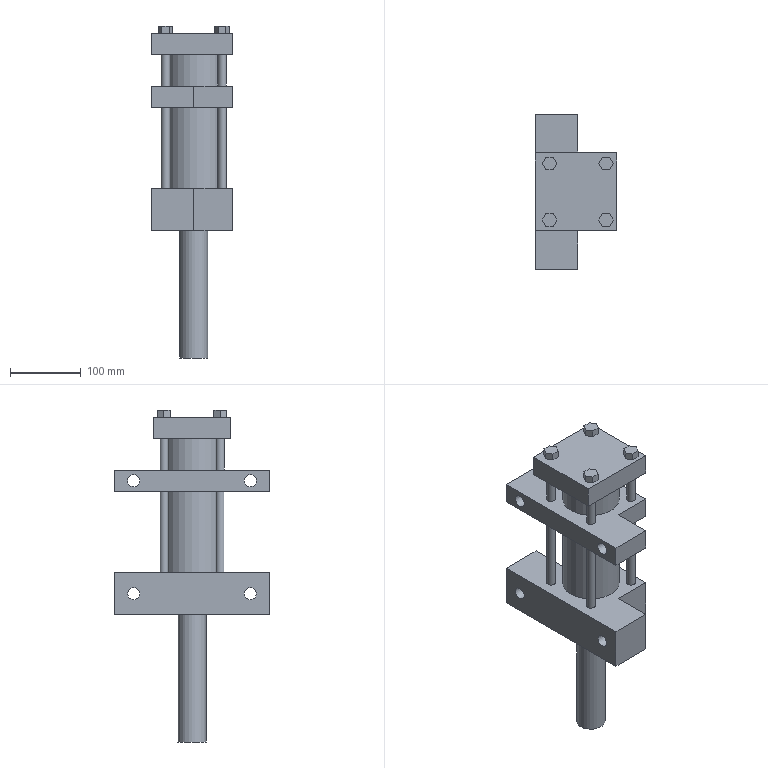Part | STEP file | solid 135 | 1 solid | 82 faces | box 115 x 220 x 470 mm | volume 3142718 mm3 | plane 59 | cylinder 21 | cone 2 | commonest cylinder face diameters 12 x8 26 x4 15 x2 17 x2 17.5 x2 80 x2